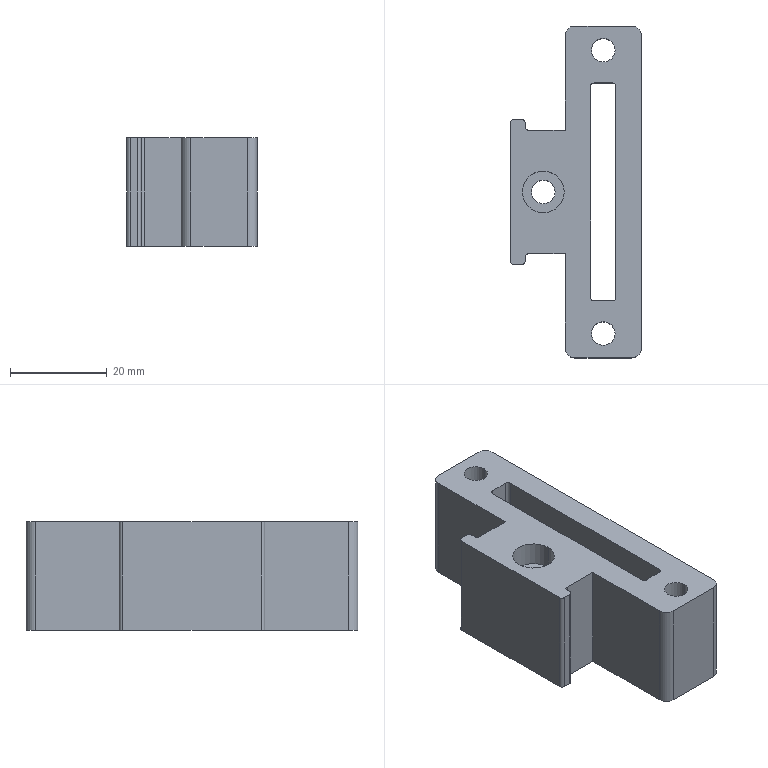Part | Creo | features DATUM PLANE 3, CURVE 2, COORDINATE SYSTEM 1, CUT 1, PROTRUSION 1, ROUND 1 | 1 solid | 41 faces | box 27 x 68.5 x 22.5 mm | volume 24185 mm3 | cylinder 22 | plane 19 | commonest cylinder face diameters 1.5 x10 4.88 x6 4 x4 8.617 x2
STEP:
#1=CARTESIAN_POINT('',(0.,0.,0.));
#2=DIRECTION('',(0.,0.,1.));
#3=DIRECTION('',(1.,0.,0.));
#4=AXIS2_PLACEMENT_3D('',#1,#2,#3);
#5=CARTESIAN_POINT('',(11.5,34.25,0.));
#6=VERTEX_POINT('',#5);
#7=CARTESIAN_POINT('',(13.5,32.25,0.));
#8=VERTEX_POINT('',#7);
#9=CARTESIAN_POINT('',(11.5,32.25,0.));
#10=DIRECTION('',(0.,0.,-1.));
#11=DIRECTION('',(0.,1.,0.));
#12=AXIS2_PLACEMENT_3D('',#9,#10,#11);
#13=CIRCLE('',#12,2.);
#14=EDGE_CURVE('',#6,#8,#13,.T.);
#15=ORIENTED_EDGE('',*,*,#14,.F.);
#16=CARTESIAN_POINT('',(-0.25,34.25,0.));
#17=VERTEX_POINT('',#16);
#18=CARTESIAN_POINT('',(11.5,34.25,0.));
#19=DIRECTION('',(-1.,0.,0.));
#20=VECTOR('',#19,11.75);
#21=LINE('',#18,#20);
#22=EDGE_CURVE('',#6,#17,#21,.T.);
#23=ORIENTED_EDGE('',*,*,#22,.T.);
#24=CARTESIAN_POINT('',(-2.25,32.25,0.));
#25=VERTEX_POINT('',#24);
#26=CARTESIAN_POINT('',(-0.25,32.25,0.));
#27=DIRECTION('',(0.,0.,-1.));
#28=DIRECTION('',(-1.,0.,0.));
#29=AXIS2_PLACEMENT_3D('',#26,#27,#28);
#30=CIRCLE('',#29,2.);
#31=EDGE_CURVE('',#25,#17,#30,.T.);
#32=ORIENTED_EDGE('',*,*,#31,.F.);
#33=CARTESIAN_POINT('',(-2.25,12.75,0.));
#34=VERTEX_POINT('',#33);
#35=CARTESIAN_POINT('',(-2.25,32.25,0.));
#36=DIRECTION('',(0.,-1.,0.));
#37=VECTOR('',#36,19.5);
#38=LINE('',#35,#37);
#39=EDGE_CURVE('',#25,#34,#38,.T.);
#40=ORIENTED_EDGE('',*,*,#39,.T.);
#41=CARTESIAN_POINT('',(-9.75,12.75,0.));
#42=VERTEX_POINT('',#41);
#43=CARTESIAN_POINT('',(-2.25,12.75,0.));
#44=DIRECTION('',(-1.,0.,0.));
#45=VECTOR('',#44,7.5);
#46=LINE('',#43,#45);
#47=EDGE_CURVE('',#34,#42,#46,.T.);
#48=ORIENTED_EDGE('',*,*,#47,.T.);
#49=CARTESIAN_POINT('',(-10.5,13.5,0.));
#50=VERTEX_POINT('',#49);
#51=CARTESIAN_POINT('',(-9.75,13.5,0.));
#52=DIRECTION('',(0.,0.,-1.));
#53=DIRECTION('',(0.,-1.,0.));
#54=AXIS2_PLACEMENT_3D('',#51,#52,#53);
#55=CIRCLE('',#54,0.75);
#56=EDGE_CURVE('',#42,#50,#55,.T.);
#57=ORIENTED_EDGE('',*,*,#56,.T.);
#58=CARTESIAN_POINT('',(-10.5,14.25,0.));
#59=VERTEX_POINT('',#58);
#60=CARTESIAN_POINT('',(-10.5,13.5,0.));
#61=DIRECTION('',(0.,1.,0.));
#62=VECTOR('',#61,0.75);
#63=LINE('',#60,#62);
#64=EDGE_CURVE('',#50,#59,#63,.T.);
#65=ORIENTED_EDGE('',*,*,#64,.T.);
#66=CARTESIAN_POINT('',(-11.25,15.,0.));
#67=VERTEX_POINT('',#66);
#68=CARTESIAN_POINT('',(-11.25,14.25,0.));
#69=DIRECTION('',(0.,0.,1.));
#70=DIRECTION('',(1.,0.,0.));
#71=AXIS2_PLACEMENT_3D('',#68,#69,#70);
#72=CIRCLE('',#71,0.75);
#73=EDGE_CURVE('',#59,#67,#72,.T.);
#74=ORIENTED_EDGE('',*,*,#73,.T.);
#75=CARTESIAN_POINT('',(-12.75,15.,0.));
#76=VERTEX_POINT('',#75);
#77=CARTESIAN_POINT('',(-11.25,15.,0.));
#78=DIRECTION('',(-1.,0.,0.));
#79=VECTOR('',#78,1.5);
#80=LINE('',#77,#79);
#81=EDGE_CURVE('',#67,#76,#80,.T.);
#82=ORIENTED_EDGE('',*,*,#81,.T.);
#83=CARTESIAN_POINT('',(-13.5,14.25,0.));
#84=VERTEX_POINT('',#83);
#85=CARTESIAN_POINT('',(-12.75,14.25,0.));
#86=DIRECTION('',(0.,0.,1.));
#87=DIRECTION('',(0.,1.,0.));
#88=AXIS2_PLACEMENT_3D('',#85,#86,#87);
#89=CIRCLE('',#88,0.75);
#90=EDGE_CURVE('',#76,#84,#89,.T.);
#91=ORIENTED_EDGE('',*,*,#90,.T.);
#92=CARTESIAN_POINT('',(-13.5,-14.25,0.));
#93=VERTEX_POINT('',#92);
#94=CARTESIAN_POINT('',(-13.5,14.25,0.));
#95=DIRECTION('',(0.,-1.,0.));
#96=VECTOR('',#95,28.5);
#97=LINE('',#94,#96);
#98=EDGE_CURVE('',#84,#93,#97,.T.);
#99=ORIENTED_EDGE('',*,*,#98,.T.);
#100=CARTESIAN_POINT('',(-12.75,-15.,0.));
#101=VERTEX_POINT('',#100);
#102=CARTESIAN_POINT('',(-12.75,-14.25,0.));
#103=DIRECTION('',(0.,0.,1.));
#104=DIRECTION('',(-1.,0.,0.));
#105=AXIS2_PLACEMENT_3D('',#102,#103,#104);
#106=CIRCLE('',#105,0.75);
#107=EDGE_CURVE('',#93,#101,#106,.T.);
#108=ORIENTED_EDGE('',*,*,#107,.T.);
#109=CARTESIAN_POINT('',(-11.25,-15.,0.));
#110=VERTEX_POINT('',#109);
#111=CARTESIAN_POINT('',(-12.75,-15.,0.));
#112=DIRECTION('',(1.,0.,0.));
#113=VECTOR('',#112,1.5);
#114=LINE('',#111,#113);
#115=EDGE_CURVE('',#101,#110,#114,.T.);
#116=ORIENTED_EDGE('',*,*,#115,.T.);
#117=CARTESIAN_POINT('',(-10.5,-14.25,0.));
#118=VERTEX_POINT('',#117);
#119=CARTESIAN_POINT('',(-11.25,-14.25,0.));
#120=DIRECTION('',(0.,0.,1.));
#121=DIRECTION('',(0.,-1.,0.));
#122=AXIS2_PLACEMENT_3D('',#119,#120,#121);
#123=CIRCLE('',#122,0.75);
#124=EDGE_CURVE('',#110,#118,#123,.T.);
#125=ORIENTED_EDGE('',*,*,#124,.T.);
#126=CARTESIAN_POINT('',(-10.5,-13.5,0.));
#127=VERTEX_POINT('',#126);
#128=CARTESIAN_POINT('',(-10.5,-14.25,0.));
#129=DIRECTION('',(0.,1.,0.));
#130=VECTOR('',#129,0.75);
#131=LINE('',#128,#130);
#132=EDGE_CURVE('',#118,#127,#131,.T.);
#133=ORIENTED_EDGE('',*,*,#132,.T.);
#134=CARTESIAN_POINT('',(-9.75,-12.75,0.));
#135=VERTEX_POINT('',#134);
#136=CARTESIAN_POINT('',(-9.75,-13.5,0.));
#137=DIRECTION('',(0.,0.,-1.));
#138=DIRECTION('',(-1.,0.,0.));
#139=AXIS2_PLACEMENT_3D('',#136,#137,#138);
#140=CIRCLE('',#139,0.75);
#141=EDGE_CURVE('',#127,#135,#140,.T.);
#142=ORIENTED_EDGE('',*,*,#141,.T.);
#143=CARTESIAN_POINT('',(-2.25,-12.75,0.));
#144=VERTEX_POINT('',#143);
#145=CARTESIAN_POINT('',(-9.75,-12.75,0.));
#146=DIRECTION('',(1.,0.,0.));
#147=VECTOR('',#146,7.5);
#148=LINE('',#145,#147);
#149=EDGE_CURVE('',#135,#144,#148,.T.);
#150=ORIENTED_EDGE('',*,*,#149,.T.);
#151=CARTESIAN_POINT('',(-2.25,-32.25,0.));
#152=VERTEX_POINT('',#151);
#153=CARTESIAN_POINT('',(-2.25,-12.75,0.));
#154=DIRECTION('',(0.,-1.,0.));
#155=VECTOR('',#154,19.5);
#156=LINE('',#153,#155);
#157=EDGE_CURVE('',#144,#152,#156,.T.);
#158=ORIENTED_EDGE('',*,*,#157,.T.);
#159=CARTESIAN_POINT('',(-0.25,-34.25,0.));
#160=VERTEX_POINT('',#159);
#161=CARTESIAN_POINT('',(-0.25,-32.25,0.));
#162=DIRECTION('',(0.,0.,-1.));
#163=DIRECTION('',(0.,-1.,0.));
#164=AXIS2_PLACEMENT_3D('',#161,#162,#163);
#165=CIRCLE('',#164,2.);
#166=EDGE_CURVE('',#160,#152,#165,.T.);
#167=ORIENTED_EDGE('',*,*,#166,.F.);
#168=CARTESIAN_POINT('',(11.5,-34.25,0.));
#169=VERTEX_POINT('',#168);
#170=CARTESIAN_POINT('',(-0.25,-34.25,0.));
#171=DIRECTION('',(1.,0.,0.));
#172=VECTOR('',#171,11.75);
#173=LINE('',#170,#172);
#174=EDGE_CURVE('',#160,#169,#173,.T.);
#175=ORIENTED_EDGE('',*,*,#174,.T.);
#176=CARTESIAN_POINT('',(13.5,-32.25,0.));
#177=VERTEX_POINT('',#176);
#178=CARTESIAN_POINT('',(11.5,-32.25,0.));
#179=DIRECTION('',(0.,0.,-1.));
#180=DIRECTION('',(1.,0.,0.));
#181=AXIS2_PLACEMENT_3D('',#178,#179,#180);
#182=CIRCLE('',#181,2.);
#183=EDGE_CURVE('',#177,#169,#182,.T.);
#184=ORIENTED_EDGE('',*,*,#183,.F.);
#185=CARTESIAN_POINT('',(13.5,-32.25,0.));
#186=DIRECTION('',(0.,1.,0.));
#187=VECTOR('',#186,64.5);
#188=LINE('',#185,#187);
#189=EDGE_CURVE('',#177,#8,#188,.T.);
#190=ORIENTED_EDGE('',*,*,#189,.T.);
#191=EDGE_LOOP('',(#15,#23,#32,#40,#48,#57,#65,#74,#82,#91,#99,#108,#116,#125,#133,#142,#150,#158,#167,#175,#184,#190));
#192=FACE_OUTER_BOUND('',#191,.F.);
#193=CARTESIAN_POINT('',(8.065,29.25,0.));
#194=VERTEX_POINT('',#193);
#195=CARTESIAN_POINT('',(3.185,29.25,0.));
#196=VERTEX_POINT('',#195);
#197=CARTESIAN_POINT('',(5.625,29.25,0.));
#198=DIRECTION('',(0.,0.,-1.));
#199=DIRECTION('',(1.,0.,0.));
#200=AXIS2_PLACEMENT_3D('',#197,#198,#199);
#201=CIRCLE('',#200,2.44);
#202=EDGE_CURVE('',#194,#196,#201,.T.);
#203=ORIENTED_EDGE('',*,*,#202,.T.);
#204=CARTESIAN_POINT('',(5.625,29.25,0.));
#205=DIRECTION('',(0.,0.,-1.));
#206=DIRECTION('',(-1.,0.,0.));
#207=AXIS2_PLACEMENT_3D('',#204,#205,#206);
#208=CIRCLE('',#207,2.44);
#209=EDGE_CURVE('',#196,#194,#208,.T.);
#210=ORIENTED_EDGE('',*,*,#209,.T.);
#211=EDGE_LOOP('',(#203,#210));
#212=FACE_BOUND('',#211,.F.);
#213=CARTESIAN_POINT('',(8.065,-29.25,0.));
#214=VERTEX_POINT('',#213);
#215=CARTESIAN_POINT('',(3.185,-29.25,0.));
#216=VERTEX_POINT('',#215);
#217=CARTESIAN_POINT('',(5.625,-29.25,0.));
#218=DIRECTION('',(0.,0.,-1.));
#219=DIRECTION('',(1.,0.,0.));
#220=AXIS2_PLACEMENT_3D('',#217,#218,#219);
#221=CIRCLE('',#220,2.44);
#222=EDGE_CURVE('',#214,#216,#221,.T.);
#223=ORIENTED_EDGE('',*,*,#222,.T.);
#224=CARTESIAN_POINT('',(5.625,-29.25,0.));
#225=DIRECTION('',(0.,0.,-1.));
#226=DIRECTION('',(-1.,0.,0.));
#227=AXIS2_PLACEMENT_3D('',#224,#225,#226);
#228=CIRCLE('',#227,2.44);
#229=EDGE_CURVE('',#216,#214,#228,.T.);
#230=ORIENTED_EDGE('',*,*,#229,.T.);
#231=EDGE_LOOP('',(#223,#230));
#232=FACE_BOUND('',#231,.F.);
#233=CARTESIAN_POINT('',(3.,21.75,0.));
#234=VERTEX_POINT('',#233);
#235=CARTESIAN_POINT('',(3.75,22.5,0.));
#236=VERTEX_POINT('',#235);
#237=CARTESIAN_POINT('',(3.75,21.75,0.));
#238=DIRECTION('',(0.,0.,-1.));
#239=DIRECTION('',(-1.,0.,0.));
#240=AXIS2_PLACEMENT_3D('',#237,#238,#239);
#241=CIRCLE('',#240,0.75);
#242=EDGE_CURVE('',#234,#236,#241,.T.);
#243=ORIENTED_EDGE('',*,*,#242,.T.);
#244=CARTESIAN_POINT('',(7.5,22.5,0.));
#245=VERTEX_POINT('',#244);
#246=CARTESIAN_POINT('',(3.75,22.5,0.));
#247=DIRECTION('',(1.,0.,0.));
#248=VECTOR('',#247,3.75);
#249=LINE('',#246,#248);
#250=EDGE_CURVE('',#236,#245,#249,.T.);
#251=ORIENTED_EDGE('',*,*,#250,.T.);
#252=CARTESIAN_POINT('',(8.25,21.75,0.));
#253=VERTEX_POINT('',#252);
#254=CARTESIAN_POINT('',(7.5,21.75,0.));
#255=DIRECTION('',(0.,0.,-1.));
#256=DIRECTION('',(0.,1.,0.));
#257=AXIS2_PLACEMENT_3D('',#254,#255,#256);
#258=CIRCLE('',#257,0.75);
#259=EDGE_CURVE('',#245,#253,#258,.T.);
#260=ORIENTED_EDGE('',*,*,#259,.T.);
#261=CARTESIAN_POINT('',(8.25,-21.75,0.));
#262=VERTEX_POINT('',#261);
#263=CARTESIAN_POINT('',(8.25,21.75,0.));
#264=DIRECTION('',(0.,-1.,0.));
#265=VECTOR('',#264,43.5);
#266=LINE('',#263,#265);
#267=EDGE_CURVE('',#253,#262,#266,.T.);
#268=ORIENTED_EDGE('',*,*,#267,.T.);
#269=CARTESIAN_POINT('',(7.5,-22.5,0.));
#270=VERTEX_POINT('',#269);
#271=CARTESIAN_POINT('',(7.5,-21.75,0.));
#272=DIRECTION('',(0.,0.,-1.));
#273=DIRECTION('',(1.,0.,0.));
#274=AXIS2_PLACEMENT_3D('',#271,#272,#273);
#275=CIRCLE('',#274,0.75);
#276=EDGE_CURVE('',#262,#270,#275,.T.);
#277=ORIENTED_EDGE('',*,*,#276,.T.);
#278=CARTESIAN_POINT('',(3.75,-22.5,0.));
#279=VERTEX_POINT('',#278);
#280=CARTESIAN_POINT('',(7.5,-22.5,0.));
#281=DIRECTION('',(-1.,0.,0.));
#282=VECTOR('',#281,3.75);
#283=LINE('',#280,#282);
#284=EDGE_CURVE('',#270,#279,#283,.T.);
#285=ORIENTED_EDGE('',*,*,#284,.T.);
#286=CARTESIAN_POINT('',(3.,-21.75,0.));
#287=VERTEX_POINT('',#286);
#288=CARTESIAN_POINT('',(3.75,-21.75,0.));
#289=DIRECTION('',(0.,0.,-1.));
#290=DIRECTION('',(0.,-1.,0.));
#291=AXIS2_PLACEMENT_3D('',#288,#289,#290);
#292=CIRCLE('',#291,0.75);
#293=EDGE_CURVE('',#279,#287,#292,.T.);
#294=ORIENTED_EDGE('',*,*,#293,.T.);
#295=CARTESIAN_POINT('',(3.,-21.75,0.));
#296=DIRECTION('',(0.,1.,0.));
#297=VECTOR('',#296,43.5);
#298=LINE('',#295,#297);
#299=EDGE_CURVE('',#287,#234,#298,.T.);
#300=ORIENTED_EDGE('',*,*,#299,.T.);
#301=EDGE_LOOP('',(#243,#251,#260,#268,#277,#285,#294,#300));
#302=FACE_BOUND('',#301,.F.);
#303=CARTESIAN_POINT('',(-4.31,0.,0.));
#304=VERTEX_POINT('',#303);
#305=CARTESIAN_POINT('',(-9.19,0.,0.));
#306=VERTEX_POINT('',#305);
#307=CARTESIAN_POINT('',(-6.75,0.,0.));
#308=DIRECTION('',(0.,0.,-1.));
#309=DIRECTION('',(1.,0.,0.));
#310=AXIS2_PLACEMENT_3D('',#307,#308,#309);
#311=CIRCLE('',#310,2.44);
#312=EDGE_CURVE('',#304,#306,#311,.T.);
#313=ORIENTED_EDGE('',*,*,#312,.T.);
#314=CARTESIAN_POINT('',(-6.75,0.,0.));
#315=DIRECTION('',(0.,0.,-1.));
#316=DIRECTION('',(-1.,0.,0.));
#317=AXIS2_PLACEMENT_3D('',#314,#315,#316);
#318=CIRCLE('',#317,2.44);
#319=EDGE_CURVE('',#306,#304,#318,.T.);
#320=ORIENTED_EDGE('',*,*,#319,.T.);
#321=EDGE_LOOP('',(#313,#320));
#322=FACE_BOUND('',#321,.F.);
#323=CARTESIAN_POINT('',(0.,0.,0.));
#324=DIRECTION('',(0.,0.,1.));
#325=DIRECTION('',(1.,0.,0.));
#326=AXIS2_PLACEMENT_3D('',#323,#324,#325);
#327=PLANE('',#326);
#328=ADVANCED_FACE('',(#192,#212,#232,#302,#322),#327,.F.);
#329=CARTESIAN_POINT('',(-9.19,0.,17.5));
#330=VERTEX_POINT('',#329);
#331=CARTESIAN_POINT('',(-4.31,0.,17.5));
#332=VERTEX_POINT('',#331);
#333=CARTESIAN_POINT('',(-6.75,0.,17.5));
#334=DIRECTION('',(0.,0.,1.));
#335=DIRECTION('',(-1.,0.,0.));
#336=AXIS2_PLACEMENT_3D('',#333,#334,#335);
#337=CIRCLE('',#336,2.44);
#338=EDGE_CURVE('',#330,#332,#337,.T.);
#339=ORIENTED_EDGE('',*,*,#338,.F.);
#340=CARTESIAN_POINT('',(-9.19,0.,0.));
#341=DIRECTION('',(0.,0.,1.));
#342=VECTOR('',#341,17.5);
#343=LINE('',#340,#342);
#344=EDGE_CURVE('',#306,#330,#343,.T.);
#345=ORIENTED_EDGE('',*,*,#344,.F.);
#346=ORIENTED_EDGE('',*,*,#312,.F.);
#347=CARTESIAN_POINT('',(-4.31,0.,0.));
#348=DIRECTION('',(0.,0.,1.));
#349=VECTOR('',#348,17.5);
#350=LINE('',#347,#349);
#351=EDGE_CURVE('',#304,#332,#350,.T.);
#352=ORIENTED_EDGE('',*,*,#351,.T.);
#353=EDGE_LOOP('',(#339,#345,#346,#352));
#354=FACE_OUTER_BOUND('',#353,.F.);
#355=CARTESIAN_POINT('',(-6.75,0.,0.));
#356=DIRECTION('',(0.,0.,1.));
#357=DIRECTION('',(1.,0.,0.));
#358=AXIS2_PLACEMENT_3D('',#355,#356,#357);
#359=CYLINDRICAL_SURFACE('',#358,2.44);
#360=ADVANCED_FACE('',(#354),#359,.F.);
#361=CARTESIAN_POINT('',(-2.441,0.,17.5));
#362=VERTEX_POINT('',#361);
#363=CARTESIAN_POINT('',(-11.059,0.,17.5));
#364=VERTEX_POINT('',#363);
#365=CARTESIAN_POINT('',(-6.75,0.,17.5));
#366=DIRECTION('',(0.,0.,1.));
#367=DIRECTION('',(1.,0.,0.));
#368=AXIS2_PLACEMENT_3D('',#365,#366,#367);
#369=CIRCLE('',#368,4.309);
#370=EDGE_CURVE('',#362,#364,#369,.T.);
#371=ORIENTED_EDGE('',*,*,#370,.F.);
#372=CARTESIAN_POINT('',(-6.75,0.,17.5));
#373=DIRECTION('',(0.,0.,1.));
#374=DIRECTION('',(-1.,0.,0.));
#375=AXIS2_PLACEMENT_3D('',#372,#373,#374);
#376=CIRCLE('',#375,4.309);
#377=EDGE_CURVE('',#364,#362,#376,.T.);
#378=ORIENTED_EDGE('',*,*,#377,.F.);
#379=EDGE_LOOP('',(#371,#378));
#380=FACE_OUTER_BOUND('',#379,.F.);
#381=ORIENTED_EDGE('',*,*,#338,.T.);
#382=CARTESIAN_POINT('',(-6.75,0.,17.5));
#383=DIRECTION('',(0.,0.,1.));
#384=DIRECTION('',(1.,0.,0.));
#385=AXIS2_PLACEMENT_3D('',#382,#383,#384);
#386=CIRCLE('',#385,2.44);
#387=EDGE_CURVE('',#332,#330,#386,.T.);
#388=ORIENTED_EDGE('',*,*,#387,.T.);
#389=EDGE_LOOP('',(#381,#388));
#390=FACE_BOUND('',#389,.F.);
#391=CARTESIAN_POINT('',(0.,0.,17.5));
#392=DIRECTION('',(0.,0.,1.));
#393=DIRECTION('',(1.,0.,0.));
#394=AXIS2_PLACEMENT_3D('',#391,#392,#393);
#395=PLANE('',#394);
#396=ADVANCED_FACE('',(#380,#390),#395,.T.);
#397=CARTESIAN_POINT('',(-2.441,0.,22.5));
#398=VERTEX_POINT('',#397);
#399=CARTESIAN_POINT('',(-11.059,0.,22.5));
#400=VERTEX_POINT('',#399);
#401=CARTESIAN_POINT('',(-6.75,0.,22.5));
#402=DIRECTION('',(0.,0.,1.));
#403=DIRECTION('',(1.,0.,0.));
#404=AXIS2_PLACEMENT_3D('',#401,#402,#403);
#405=CIRCLE('',#404,4.309);
#406=EDGE_CURVE('',#398,#400,#405,.T.);
#407=ORIENTED_EDGE('',*,*,#406,.F.);
#408=CARTESIAN_POINT('',(-2.441,0.,22.5));
#409=DIRECTION('',(0.,0.,-1.));
#410=VECTOR('',#409,5.);
#411=LINE('',#408,#410);
#412=EDGE_CURVE('',#398,#362,#411,.T.);
#413=ORIENTED_EDGE('',*,*,#412,.T.);
#414=ORIENTED_EDGE('',*,*,#370,.T.);
#415=CARTESIAN_POINT('',(-11.059,0.,22.5));
#416=DIRECTION('',(0.,0.,-1.));
#417=VECTOR('',#416,5.);
#418=LINE('',#415,#417);
#419=EDGE_CURVE('',#400,#364,#418,.T.);
#420=ORIENTED_EDGE('',*,*,#419,.F.);
#421=EDGE_LOOP('',(#407,#413,#414,#420));
#422=FACE_OUTER_BOUND('',#421,.F.);
#423=CARTESIAN_POINT('',(-6.75,0.,22.5));
#424=DIRECTION('',(0.,0.,1.));
#425=DIRECTION('',(1.,0.,0.));
#426=AXIS2_PLACEMENT_3D('',#423,#424,#425);
#427=CYLINDRICAL_SURFACE('',#426,4.309);
#428=ADVANCED_FACE('',(#422),#427,.F.);
#429=CARTESIAN_POINT('',(13.5,32.25,22.5));
#430=VERTEX_POINT('',#429);
#431=CARTESIAN_POINT('',(11.5,34.25,22.5));
#432=VERTEX_POINT('',#431);
#433=CARTESIAN_POINT('',(11.5,32.25,22.5));
#434=DIRECTION('',(0.,0.,1.));
#435=DIRECTION('',(1.,0.,0.));
#436=AXIS2_PLACEMENT_3D('',#433,#434,#435);
#437=CIRCLE('',#436,2.);
#438=EDGE_CURVE('',#430,#432,#437,.T.);
#439=ORIENTED_EDGE('',*,*,#438,.F.);
#440=CARTESIAN_POINT('',(13.5,-32.25,22.5));
#441=VERTEX_POINT('',#440);
#442=CARTESIAN_POINT('',(13.5,-32.25,22.5));
#443=DIRECTION('',(0.,1.,0.));
#444=VECTOR('',#443,64.5);
#445=LINE('',#442,#444);
#446=EDGE_CURVE('',#441,#430,#445,.T.);
#447=ORIENTED_EDGE('',*,*,#446,.F.);
#448=CARTESIAN_POINT('',(11.5,-34.25,22.5));
#449=VERTEX_POINT('',#448);
#450=CARTESIAN_POINT('',(11.5,-32.25,22.5));
#451=DIRECTION('',(0.,0.,1.));
#452=DIRECTION('',(0.,-1.,0.));
#453=AXIS2_PLACEMENT_3D('',#450,#451,#452);
#454=CIRCLE('',#453,2.);
#455=EDGE_CURVE('',#449,#441,#454,.T.);
#456=ORIENTED_EDGE('',*,*,#455,.F.);
#457=CARTESIAN_POINT('',(-0.25,-34.25,22.5));
#458=VERTEX_POINT('',#457);
#459=CARTESIAN_POINT('',(-0.25,-34.25,22.5));
#460=DIRECTION('',(1.,0.,0.));
#461=VECTOR('',#460,11.75);
#462=LINE('',#459,#461);
#463=EDGE_CURVE('',#458,#449,#462,.T.);
#464=ORIENTED_EDGE('',*,*,#463,.F.);
#465=CARTESIAN_POINT('',(-2.25,-32.25,22.5));
#466=VERTEX_POINT('',#465);
#467=CARTESIAN_POINT('',(-0.25,-32.25,22.5));
#468=DIRECTION('',(0.,0.,1.));
#469=DIRECTION('',(-1.,0.,0.));
#470=AXIS2_PLACEMENT_3D('',#467,#468,#469);
#471=CIRCLE('',#470,2.);
#472=EDGE_CURVE('',#466,#458,#471,.T.);
#473=ORIENTED_EDGE('',*,*,#472,.F.);
#474=CARTESIAN_POINT('',(-2.25,-12.75,22.5));
#475=VERTEX_POINT('',#474);
#476=CARTESIAN_POINT('',(-2.25,-12.75,22.5));
#477=DIRECTION('',(0.,-1.,0.));
#478=VECTOR('',#477,19.5);
#479=LINE('',#476,#478);
#480=EDGE_CURVE('',#475,#466,#479,.T.);
#481=ORIENTED_EDGE('',*,*,#480,.F.);
#482=CARTESIAN_POINT('',(-9.75,-12.75,22.5));
#483=VERTEX_POINT('',#482);
#484=CARTESIAN_POINT('',(-9.75,-12.75,22.5));
#485=DIRECTION('',(1.,0.,0.));
#486=VECTOR('',#485,7.5);
#487=LINE('',#484,#486);
#488=EDGE_CURVE('',#483,#475,#487,.T.);
#489=ORIENTED_EDGE('',*,*,#488,.F.);
#490=CARTESIAN_POINT('',(-10.5,-13.5,22.5));
#491=VERTEX_POINT('',#490);
#492=CARTESIAN_POINT('',(-9.75,-13.5,22.5));
#493=DIRECTION('',(0.,0.,-1.));
#494=DIRECTION('',(-1.,0.,0.));
#495=AXIS2_PLACEMENT_3D('',#492,#493,#494);
#496=CIRCLE('',#495,0.75);
#497=EDGE_CURVE('',#491,#483,#496,.T.);
#498=ORIENTED_EDGE('',*,*,#497,.F.);
#499=CARTESIAN_POINT('',(-10.5,-14.25,22.5));
#500=VERTEX_POINT('',#499);
#501=CARTESIAN_POINT('',(-10.5,-14.25,22.5));
#502=DIRECTION('',(0.,1.,0.));
#503=VECTOR('',#502,0.75);
#504=LINE('',#501,#503);
#505=EDGE_CURVE('',#500,#491,#504,.T.);
#506=ORIENTED_EDGE('',*,*,#505,.F.);
#507=CARTESIAN_POINT('',(-11.25,-15.,22.5));
#508=VERTEX_POINT('',#507);
#509=CARTESIAN_POINT('',(-11.25,-14.25,22.5));
#510=DIRECTION('',(0.,0.,1.));
#511=DIRECTION('',(0.,-1.,0.));
#512=AXIS2_PLACEMENT_3D('',#509,#510,#511);
#513=CIRCLE('',#512,0.75);
#514=EDGE_CURVE('',#508,#500,#513,.T.);
#515=ORIENTED_EDGE('',*,*,#514,.F.);
#516=CARTESIAN_POINT('',(-12.75,-15.,22.5));
#517=VERTEX_POINT('',#516);
#518=CARTESIAN_POINT('',(-12.75,-15.,22.5));
#519=DIRECTION('',(1.,0.,0.));
#520=VECTOR('',#519,1.5);
#521=LINE('',#518,#520);
#522=EDGE_CURVE('',#517,#508,#521,.T.);
#523=ORIENTED_EDGE('',*,*,#522,.F.);
#524=CARTESIAN_POINT('',(-13.5,-14.25,22.5));
#525=VERTEX_POINT('',#524);
#526=CARTESIAN_POINT('',(-12.75,-14.25,22.5));
#527=DIRECTION('',(0.,0.,1.));
#528=DIRECTION('',(-1.,0.,0.));
#529=AXIS2_PLACEMENT_3D('',#526,#527,#528);
#530=CIRCLE('',#529,0.75);
#531=EDGE_CURVE('',#525,#517,#530,.T.);
#532=ORIENTED_EDGE('',*,*,#531,.F.);
#533=CARTESIAN_POINT('',(-13.5,14.25,22.5));
#534=VERTEX_POINT('',#533);
#535=CARTESIAN_POINT('',(-13.5,14.25,22.5));
#536=DIRECTION('',(0.,-1.,0.));
#537=VECTOR('',#536,28.5);
#538=LINE('',#535,#537);
#539=EDGE_CURVE('',#534,#525,#538,.T.);
#540=ORIENTED_EDGE('',*,*,#539,.F.);
#541=CARTESIAN_POINT('',(-12.75,15.,22.5));
#542=VERTEX_POINT('',#541);
#543=CARTESIAN_POINT('',(-12.75,14.25,22.5));
#544=DIRECTION('',(0.,0.,1.));
#545=DIRECTION('',(0.,1.,0.));
#546=AXIS2_PLACEMENT_3D('',#543,#544,#545);
#547=CIRCLE('',#546,0.75);
#548=EDGE_CURVE('',#542,#534,#547,.T.);
#549=ORIENTED_EDGE('',*,*,#548,.F.);
#550=CARTESIAN_POINT('',(-11.25,15.,22.5));
#551=VERTEX_POINT('',#550);
#552=CARTESIAN_POINT('',(-11.25,15.,22.5));
#553=DIRECTION('',(-1.,0.,0.));
#554=VECTOR('',#553,1.5);
#555=LINE('',#552,#554);
#556=EDGE_CURVE('',#551,#542,#555,.T.);
#557=ORIENTED_EDGE('',*,*,#556,.F.);
#558=CARTESIAN_POINT('',(-10.5,14.25,22.5));
#559=VERTEX_POINT('',#558);
#560=CARTESIAN_POINT('',(-11.25,14.25,22.5));
#561=DIRECTION('',(0.,0.,1.));
#562=DIRECTION('',(1.,0.,0.));
#563=AXIS2_PLACEMENT_3D('',#560,#561,#562);
#564=CIRCLE('',#563,0.75);
#565=EDGE_CURVE('',#559,#551,#564,.T.);
#566=ORIENTED_EDGE('',*,*,#565,.F.);
#567=CARTESIAN_POINT('',(-10.5,13.5,22.5));
#568=VERTEX_POINT('',#567);
#569=CARTESIAN_POINT('',(-10.5,13.5,22.5));
#570=DIRECTION('',(0.,1.,0.));
#571=VECTOR('',#570,0.75);
#572=LINE('',#569,#571);
#573=EDGE_CURVE('',#568,#559,#572,.T.);
#574=ORIENTED_EDGE('',*,*,#573,.F.);
#575=CARTESIAN_POINT('',(-9.75,12.75,22.5));
#576=VERTEX_POINT('',#575);
#577=CARTESIAN_POINT('',(-9.75,13.5,22.5));
#578=DIRECTION('',(0.,0.,-1.));
#579=DIRECTION('',(0.,-1.,0.));
#580=AXIS2_PLACEMENT_3D('',#577,#578,#579);
#581=CIRCLE('',#580,0.75);
#582=EDGE_CURVE('',#576,#568,#581,.T.);
#583=ORIENTED_EDGE('',*,*,#582,.F.);
#584=CARTESIAN_POINT('',(-2.25,12.75,22.5));
#585=VERTEX_POINT('',#584);
#586=CARTESIAN_POINT('',(-2.25,12.75,22.5));
#587=DIRECTION('',(-1.,0.,0.));
#588=VECTOR('',#587,7.5);
#589=LINE('',#586,#588);
#590=EDGE_CURVE('',#585,#576,#589,.T.);
#591=ORIENTED_EDGE('',*,*,#590,.F.);
#592=CARTESIAN_POINT('',(-2.25,32.25,22.5));
#593=VERTEX_POINT('',#592);
#594=CARTESIAN_POINT('',(-2.25,32.25,22.5));
#595=DIRECTION('',(0.,-1.,0.));
#596=VECTOR('',#595,19.5);
#597=LINE('',#594,#596);
#598=EDGE_CURVE('',#593,#585,#597,.T.);
#599=ORIENTED_EDGE('',*,*,#598,.F.);
#600=CARTESIAN_POINT('',(-0.25,34.25,22.5));
#601=VERTEX_POINT('',#600);
#602=CARTESIAN_POINT('',(-0.25,32.25,22.5));
#603=DIRECTION('',(0.,0.,1.));
#604=DIRECTION('',(0.,1.,0.));
#605=AXIS2_PLACEMENT_3D('',#602,#603,#604);
#606=CIRCLE('',#605,2.);
#607=EDGE_CURVE('',#601,#593,#606,.T.);
#608=ORIENTED_EDGE('',*,*,#607,.F.);
#609=CARTESIAN_POINT('',(11.5,34.25,22.5));
#610=DIRECTION('',(-1.,0.,0.));
#611=VECTOR('',#610,11.75);
#612=LINE('',#609,#611);
#613=EDGE_CURVE('',#432,#601,#612,.T.);
#614=ORIENTED_EDGE('',*,*,#613,.F.);
#615=EDGE_LOOP('',(#439,#447,#456,#464,#473,#481,#489,#498,#506,#515,#523,#532,#540,#549,#557,#566,#574,#583,#591,#599,#608,#614));
#616=FACE_OUTER_BOUND('',#615,.F.);
#617=CARTESIAN_POINT('',(8.065,-29.25,22.5));
#618=VERTEX_POINT('',#617);
#619=CARTESIAN_POINT('',(3.185,-29.25,22.5));
#620=VERTEX_POINT('',#619);
#621=CARTESIAN_POINT('',(5.625,-29.25,22.5));
#622=DIRECTION('',(0.,0.,-1.));
#623=DIRECTION('',(1.,0.,0.));
#624=AXIS2_PLACEMENT_3D('',#621,#622,#623);
#625=CIRCLE('',#624,2.44);
#626=EDGE_CURVE('',#618,#620,#625,.T.);
#627=ORIENTED_EDGE('',*,*,#626,.F.);
#628=CARTESIAN_POINT('',(5.625,-29.25,22.5));
#629=DIRECTION('',(0.,0.,-1.));
#630=DIRECTION('',(-1.,0.,0.));
#631=AXIS2_PLACEMENT_3D('',#628,#629,#630);
#632=CIRCLE('',#631,2.44);
#633=EDGE_CURVE('',#620,#618,#632,.T.);
#634=ORIENTED_EDGE('',*,*,#633,.F.);
#635=EDGE_LOOP('',(#627,#634));
#636=FACE_BOUND('',#635,.F.);
#637=CARTESIAN_POINT('',(3.,21.75,22.5));
#638=VERTEX_POINT('',#637);
#639=CARTESIAN_POINT('',(3.75,22.5,22.5));
#640=VERTEX_POINT('',#639);
#641=CARTESIAN_POINT('',(3.75,21.75,22.5));
#642=DIRECTION('',(0.,0.,-1.));
#643=DIRECTION('',(-1.,0.,0.));
#644=AXIS2_PLACEMENT_3D('',#641,#642,#643);
#645=CIRCLE('',#644,0.75);
#646=EDGE_CURVE('',#638,#640,#645,.T.);
#647=ORIENTED_EDGE('',*,*,#646,.F.);
#648=CARTESIAN_POINT('',(3.,-21.75,22.5));
#649=VERTEX_POINT('',#648);
#650=CARTESIAN_POINT('',(3.,-21.75,22.5));
#651=DIRECTION('',(0.,1.,0.));
#652=VECTOR('',#651,43.5);
#653=LINE('',#650,#652);
#654=EDGE_CURVE('',#649,#638,#653,.T.);
#655=ORIENTED_EDGE('',*,*,#654,.F.);
#656=CARTESIAN_POINT('',(3.75,-22.5,22.5));
#657=VERTEX_POINT('',#656);
#658=CARTESIAN_POINT('',(3.75,-21.75,22.5));
#659=DIRECTION('',(0.,0.,-1.));
#660=DIRECTION('',(0.,-1.,0.));
#661=AXIS2_PLACEMENT_3D('',#658,#659,#660);
#662=CIRCLE('',#661,0.75);
#663=EDGE_CURVE('',#657,#649,#662,.T.);
#664=ORIENTED_EDGE('',*,*,#663,.F.);
#665=CARTESIAN_POINT('',(7.5,-22.5,22.5));
#666=VERTEX_POINT('',#665);
#667=CARTESIAN_POINT('',(7.5,-22.5,22.5));
#668=DIRECTION('',(-1.,0.,0.));
#669=VECTOR('',#668,3.75);
#670=LINE('',#667,#669);
#671=EDGE_CURVE('',#666,#657,#670,.T.);
#672=ORIENTED_EDGE('',*,*,#671,.F.);
#673=CARTESIAN_POINT('',(8.25,-21.75,22.5));
#674=VERTEX_POINT('',#673);
#675=CARTESIAN_POINT('',(7.5,-21.75,22.5));
#676=DIRECTION('',(0.,0.,-1.));
#677=DIRECTION('',(1.,0.,0.));
#678=AXIS2_PLACEMENT_3D('',#675,#676,#677);
#679=CIRCLE('',#678,0.75);
#680=EDGE_CURVE('',#674,#666,#679,.T.);
#681=ORIENTED_EDGE('',*,*,#680,.F.);
#682=CARTESIAN_POINT('',(8.25,21.75,22.5));
#683=VERTEX_POINT('',#682);
#684=CARTESIAN_POINT('',(8.25,21.75,22.5));
#685=DIRECTION('',(0.,-1.,0.));
#686=VECTOR('',#685,43.5);
#687=LINE('',#684,#686);
#688=EDGE_CURVE('',#683,#674,#687,.T.);
#689=ORIENTED_EDGE('',*,*,#688,.F.);
#690=CARTESIAN_POINT('',(7.5,22.5,22.5));
#691=VERTEX_POINT('',#690);
#692=CARTESIAN_POINT('',(7.5,21.75,22.5));
#693=DIRECTION('',(0.,0.,-1.));
#694=DIRECTION('',(0.,1.,0.));
#695=AXIS2_PLACEMENT_3D('',#692,#693,#694);
#696=CIRCLE('',#695,0.75);
#697=EDGE_CURVE('',#691,#683,#696,.T.);
#698=ORIENTED_EDGE('',*,*,#697,.F.);
#699=CARTESIAN_POINT('',(3.75,22.5,22.5));
#700=DIRECTION('',(1.,0.,0.));
#701=VECTOR('',#700,3.75);
#702=LINE('',#699,#701);
#703=EDGE_CURVE('',#640,#691,#702,.T.);
#704=ORIENTED_EDGE('',*,*,#703,.F.);
#705=EDGE_LOOP('',(#647,#655,#664,#672,#681,#689,#698,#704));
#706=FACE_BOUND('',#705,.F.);
#707=ORIENTED_EDGE('',*,*,#406,.T.);
#708=CARTESIAN_POINT('',(-6.75,0.,22.5));
#709=DIRECTION('',(0.,0.,1.));
#710=DIRECTION('',(-1.,0.,0.));
#711=AXIS2_PLACEMENT_3D('',#708,#709,#710);
#712=CIRCLE('',#711,4.309);
#713=EDGE_CURVE('',#400,#398,#712,.T.);
#714=ORIENTED_EDGE('',*,*,#713,.T.);
#715=EDGE_LOOP('',(#707,#714));
#716=FACE_BOUND('',#715,.F.);
#717=CARTESIAN_POINT('',(8.065,29.25,22.5));
#718=VERTEX_POINT('',#717);
#719=CARTESIAN_POINT('',(3.185,29.25,22.5));
#720=VERTEX_POINT('',#719);
#721=CARTESIAN_POINT('',(5.625,29.25,22.5));
#722=DIRECTION('',(0.,0.,-1.));
#723=DIRECTION('',(1.,0.,0.));
#724=AXIS2_PLACEMENT_3D('',#721,#722,#723);
#725=CIRCLE('',#724,2.44);
#726=EDGE_CURVE('',#718,#720,#725,.T.);
#727=ORIENTED_EDGE('',*,*,#726,.F.);
#728=CARTESIAN_POINT('',(5.625,29.25,22.5));
#729=DIRECTION('',(0.,0.,-1.));
#730=DIRECTION('',(-1.,0.,0.));
#731=AXIS2_PLACEMENT_3D('',#728,#729,#730);
#732=CIRCLE('',#731,2.44);
#733=EDGE_CURVE('',#720,#718,#732,.T.);
#734=ORIENTED_EDGE('',*,*,#733,.F.);
#735=EDGE_LOOP('',(#727,#734));
#736=FACE_BOUND('',#735,.F.);
#737=CARTESIAN_POINT('',(0.,0.,22.5));
#738=DIRECTION('',(0.,0.,1.));
#739=DIRECTION('',(1.,0.,0.));
#740=AXIS2_PLACEMENT_3D('',#737,#738,#739);
#741=PLANE('',#740);
#742=ADVANCED_FACE('',(#616,#636,#706,#716,#736),#741,.T.);
#743=ORIENTED_EDGE('',*,*,#202,.F.);
#744=CARTESIAN_POINT('',(8.065,29.25,0.));
#745=DIRECTION('',(0.,0.,1.));
#746=VECTOR('',#745,22.5);
#747=LINE('',#744,#746);
#748=EDGE_CURVE('',#194,#718,#747,.T.);
#749=ORIENTED_EDGE('',*,*,#748,.T.);
#750=ORIENTED_EDGE('',*,*,#726,.T.);
#751=CARTESIAN_POINT('',(3.185,29.25,0.));
#752=DIRECTION('',(0.,0.,1.));
#753=VECTOR('',#752,22.5);
#754=LINE('',#751,#753);
#755=EDGE_CURVE('',#196,#720,#754,.T.);
#756=ORIENTED_EDGE('',*,*,#755,.F.);
#757=EDGE_LOOP('',(#743,#749,#750,#756));
#758=FACE_OUTER_BOUND('',#757,.F.);
#759=CARTESIAN_POINT('',(5.625,29.25,0.));
#760=DIRECTION('',(0.,0.,1.));
#761=DIRECTION('',(1.,0.,0.));
#762=AXIS2_PLACEMENT_3D('',#759,#760,#761);
#763=CYLINDRICAL_SURFACE('',#762,2.44);
#764=ADVANCED_FACE('',(#758),#763,.F.);
#765=ORIENTED_EDGE('',*,*,#209,.F.);
#766=ORIENTED_EDGE('',*,*,#755,.T.);
#767=ORIENTED_EDGE('',*,*,#733,.T.);
#768=ORIENTED_EDGE('',*,*,#748,.F.);
#769=EDGE_LOOP('',(#765,#766,#767,#768));
#770=FACE_OUTER_BOUND('',#769,.F.);
#771=CARTESIAN_POINT('',(5.625,29.25,0.));
#772=DIRECTION('',(0.,0.,1.));
#773=DIRECTION('',(1.,0.,0.));
#774=AXIS2_PLACEMENT_3D('',#771,#772,#773);
#775=CYLINDRICAL_SURFACE('',#774,2.44);
#776=ADVANCED_FACE('',(#770),#775,.F.);
#777=ORIENTED_EDGE('',*,*,#222,.F.);
#778=CARTESIAN_POINT('',(8.065,-29.25,0.));
#779=DIRECTION('',(0.,0.,1.));
#780=VECTOR('',#779,22.5);
#781=LINE('',#778,#780);
#782=EDGE_CURVE('',#214,#618,#781,.T.);
#783=ORIENTED_EDGE('',*,*,#782,.T.);
#784=ORIENTED_EDGE('',*,*,#626,.T.);
#785=CARTESIAN_POINT('',(3.185,-29.25,0.));
#786=DIRECTION('',(0.,0.,1.));
#787=VECTOR('',#786,22.5);
#788=LINE('',#785,#787);
#789=EDGE_CURVE('',#216,#620,#788,.T.);
#790=ORIENTED_EDGE('',*,*,#789,.F.);
#791=EDGE_LOOP('',(#777,#783,#784,#790));
#792=FACE_OUTER_BOUND('',#791,.F.);
#793=CARTESIAN_POINT('',(5.625,-29.25,0.));
#794=DIRECTION('',(0.,0.,1.));
#795=DIRECTION('',(1.,0.,0.));
#796=AXIS2_PLACEMENT_3D('',#793,#794,#795);
#797=CYLINDRICAL_SURFACE('',#796,2.44);
#798=ADVANCED_FACE('',(#792),#797,.F.);
#799=ORIENTED_EDGE('',*,*,#229,.F.);
#800=ORIENTED_EDGE('',*,*,#789,.T.);
#801=ORIENTED_EDGE('',*,*,#633,.T.);
#802=ORIENTED_EDGE('',*,*,#782,.F.);
#803=EDGE_LOOP('',(#799,#800,#801,#802));
#804=FACE_OUTER_BOUND('',#803,.F.);
#805=CARTESIAN_POINT('',(5.625,-29.25,0.));
#806=DIRECTION('',(0.,0.,1.));
#807=DIRECTION('',(1.,0.,0.));
#808=AXIS2_PLACEMENT_3D('',#805,#806,#807);
#809=CYLINDRICAL_SURFACE('',#808,2.44);
#810=ADVANCED_FACE('',(#804),#809,.F.);
#811=ORIENTED_EDGE('',*,*,#242,.F.);
#812=CARTESIAN_POINT('',(3.,21.75,0.));
#813=DIRECTION('',(0.,0.,1.));
#814=VECTOR('',#813,22.5);
#815=LINE('',#812,#814);
#816=EDGE_CURVE('',#234,#638,#815,.T.);
#817=ORIENTED_EDGE('',*,*,#816,.T.);
#818=ORIENTED_EDGE('',*,*,#646,.T.);
#819=CARTESIAN_POINT('',(3.75,22.5,0.));
#820=DIRECTION('',(0.,0.,1.));
#821=VECTOR('',#820,22.5);
#822=LINE('',#819,#821);
#823=EDGE_CURVE('',#236,#640,#822,.T.);
#824=ORIENTED_EDGE('',*,*,#823,.F.);
#825=EDGE_LOOP('',(#811,#817,#818,#824));
#826=FACE_OUTER_BOUND('',#825,.F.);
#827=CARTESIAN_POINT('',(3.75,21.75,0.));
#828=DIRECTION('',(0.,0.,1.));
#829=DIRECTION('',(1.,0.,0.));
#830=AXIS2_PLACEMENT_3D('',#827,#828,#829);
#831=CYLINDRICAL_SURFACE('',#830,0.75);
#832=ADVANCED_FACE('',(#826),#831,.F.);
#833=ORIENTED_EDGE('',*,*,#299,.F.);
#834=CARTESIAN_POINT('',(3.,-21.75,0.));
#835=DIRECTION('',(0.,0.,1.));
#836=VECTOR('',#835,22.5);
#837=LINE('',#834,#836);
#838=EDGE_CURVE('',#287,#649,#837,.T.);
#839=ORIENTED_EDGE('',*,*,#838,.T.);
#840=ORIENTED_EDGE('',*,*,#654,.T.);
#841=ORIENTED_EDGE('',*,*,#816,.F.);
#842=EDGE_LOOP('',(#833,#839,#840,#841));
#843=FACE_OUTER_BOUND('',#842,.F.);
#844=CARTESIAN_POINT('',(3.,-21.75,0.));
#845=DIRECTION('',(1.,0.,0.));
#846=DIRECTION('',(0.,1.,0.));
#847=AXIS2_PLACEMENT_3D('',#844,#845,#846);
#848=PLANE('',#847);
#849=ADVANCED_FACE('',(#843),#848,.T.);
#850=ORIENTED_EDGE('',*,*,#293,.F.);
#851=CARTESIAN_POINT('',(3.75,-22.5,0.));
#852=DIRECTION('',(0.,0.,1.));
#853=VECTOR('',#852,22.5);
#854=LINE('',#851,#853);
#855=EDGE_CURVE('',#279,#657,#854,.T.);
#856=ORIENTED_EDGE('',*,*,#855,.T.);
#857=ORIENTED_EDGE('',*,*,#663,.T.);
#858=ORIENTED_EDGE('',*,*,#838,.F.);
#859=EDGE_LOOP('',(#850,#856,#857,#858));
#860=FACE_OUTER_BOUND('',#859,.F.);
#861=CARTESIAN_POINT('',(3.75,-21.75,0.));
#862=DIRECTION('',(0.,0.,1.));
#863=DIRECTION('',(1.,0.,0.));
#864=AXIS2_PLACEMENT_3D('',#861,#862,#863);
#865=CYLINDRICAL_SURFACE('',#864,0.75);
#866=ADVANCED_FACE('',(#860),#865,.F.);
#867=ORIENTED_EDGE('',*,*,#284,.F.);
#868=CARTESIAN_POINT('',(7.5,-22.5,0.));
#869=DIRECTION('',(0.,0.,1.));
#870=VECTOR('',#869,22.5);
#871=LINE('',#868,#870);
#872=EDGE_CURVE('',#270,#666,#871,.T.);
#873=ORIENTED_EDGE('',*,*,#872,.T.);
#874=ORIENTED_EDGE('',*,*,#671,.T.);
#875=ORIENTED_EDGE('',*,*,#855,.F.);
#876=EDGE_LOOP('',(#867,#873,#874,#875));
#877=FACE_OUTER_BOUND('',#876,.F.);
#878=CARTESIAN_POINT('',(7.5,-22.5,0.));
#879=DIRECTION('',(0.,1.,0.));
#880=DIRECTION('',(-1.,0.,0.));
#881=AXIS2_PLACEMENT_3D('',#878,#879,#880);
#882=PLANE('',#881);
#883=ADVANCED_FACE('',(#877),#882,.T.);
#884=ORIENTED_EDGE('',*,*,#276,.F.);
#885=CARTESIAN_POINT('',(8.25,-21.75,0.));
#886=DIRECTION('',(0.,0.,1.));
#887=VECTOR('',#886,22.5);
#888=LINE('',#885,#887);
#889=EDGE_CURVE('',#262,#674,#888,.T.);
#890=ORIENTED_EDGE('',*,*,#889,.T.);
#891=ORIENTED_EDGE('',*,*,#680,.T.);
#892=ORIENTED_EDGE('',*,*,#872,.F.);
#893=EDGE_LOOP('',(#884,#890,#891,#892));
#894=FACE_OUTER_BOUND('',#893,.F.);
#895=CARTESIAN_POINT('',(7.5,-21.75,0.));
#896=DIRECTION('',(0.,0.,1.));
#897=DIRECTION('',(1.,0.,0.));
#898=AXIS2_PLACEMENT_3D('',#895,#896,#897);
#899=CYLINDRICAL_SURFACE('',#898,0.75);
#900=ADVANCED_FACE('',(#894),#899,.F.);
#901=ORIENTED_EDGE('',*,*,#267,.F.);
#902=CARTESIAN_POINT('',(8.25,21.75,0.));
#903=DIRECTION('',(0.,0.,1.));
#904=VECTOR('',#903,22.5);
#905=LINE('',#902,#904);
#906=EDGE_CURVE('',#253,#683,#905,.T.);
#907=ORIENTED_EDGE('',*,*,#906,.T.);
#908=ORIENTED_EDGE('',*,*,#688,.T.);
#909=ORIENTED_EDGE('',*,*,#889,.F.);
#910=EDGE_LOOP('',(#901,#907,#908,#909));
#911=FACE_OUTER_BOUND('',#910,.F.);
#912=CARTESIAN_POINT('',(8.25,21.75,0.));
#913=DIRECTION('',(-1.,0.,0.));
#914=DIRECTION('',(0.,-1.,0.));
#915=AXIS2_PLACEMENT_3D('',#912,#913,#914);
#916=PLANE('',#915);
#917=ADVANCED_FACE('',(#911),#916,.T.);
#918=ORIENTED_EDGE('',*,*,#259,.F.);
#919=CARTESIAN_POINT('',(7.5,22.5,0.));
#920=DIRECTION('',(0.,0.,1.));
#921=VECTOR('',#920,22.5);
#922=LINE('',#919,#921);
#923=EDGE_CURVE('',#245,#691,#922,.T.);
#924=ORIENTED_EDGE('',*,*,#923,.T.);
#925=ORIENTED_EDGE('',*,*,#697,.T.);
#926=ORIENTED_EDGE('',*,*,#906,.F.);
#927=EDGE_LOOP('',(#918,#924,#925,#926));
#928=FACE_OUTER_BOUND('',#927,.F.);
#929=CARTESIAN_POINT('',(7.5,21.75,0.));
#930=DIRECTION('',(0.,0.,1.));
#931=DIRECTION('',(1.,0.,0.));
#932=AXIS2_PLACEMENT_3D('',#929,#930,#931);
#933=CYLINDRICAL_SURFACE('',#932,0.75);
#934=ADVANCED_FACE('',(#928),#933,.F.);
#935=ORIENTED_EDGE('',*,*,#250,.F.);
#936=ORIENTED_EDGE('',*,*,#823,.T.);
#937=ORIENTED_EDGE('',*,*,#703,.T.);
#938=ORIENTED_EDGE('',*,*,#923,.F.);
#939=EDGE_LOOP('',(#935,#936,#937,#938));
#940=FACE_OUTER_BOUND('',#939,.F.);
#941=CARTESIAN_POINT('',(3.75,22.5,0.));
#942=DIRECTION('',(0.,-1.,0.));
#943=DIRECTION('',(1.,0.,0.));
#944=AXIS2_PLACEMENT_3D('',#941,#942,#943);
#945=PLANE('',#944);
#946=ADVANCED_FACE('',(#940),#945,.T.);
#947=ORIENTED_EDGE('',*,*,#713,.F.);
#948=ORIENTED_EDGE('',*,*,#419,.T.);
#949=ORIENTED_EDGE('',*,*,#377,.T.);
#950=ORIENTED_EDGE('',*,*,#412,.F.);
#951=EDGE_LOOP('',(#947,#948,#949,#950));
#952=FACE_OUTER_BOUND('',#951,.F.);
#953=CARTESIAN_POINT('',(-6.75,0.,22.5));
#954=DIRECTION('',(0.,0.,1.));
#955=DIRECTION('',(1.,0.,0.));
#956=AXIS2_PLACEMENT_3D('',#953,#954,#955);
#957=CYLINDRICAL_SURFACE('',#956,4.309);
#958=ADVANCED_FACE('',(#952),#957,.F.);
#959=ORIENTED_EDGE('',*,*,#14,.T.);
#960=CARTESIAN_POINT('',(13.5,32.25,22.5));
#961=DIRECTION('',(0.,0.,-1.));
#962=VECTOR('',#961,22.5);
#963=LINE('',#960,#962);
#964=EDGE_CURVE('',#430,#8,#963,.T.);
#965=ORIENTED_EDGE('',*,*,#964,.F.);
#966=ORIENTED_EDGE('',*,*,#438,.T.);
#967=CARTESIAN_POINT('',(11.5,34.25,22.5));
#968=DIRECTION('',(0.,0.,-1.));
#969=VECTOR('',#968,22.5);
#970=LINE('',#967,#969);
#971=EDGE_CURVE('',#432,#6,#970,.T.);
#972=ORIENTED_EDGE('',*,*,#971,.T.);
#973=EDGE_LOOP('',(#959,#965,#966,#972));
#974=FACE_OUTER_BOUND('',#973,.F.);
#975=CARTESIAN_POINT('',(11.5,32.25,51.831));
#976=DIRECTION('',(0.,0.,-1.));
#977=DIRECTION('',(0.,1.,0.));
#978=AXIS2_PLACEMENT_3D('',#975,#976,#977);
#979=CYLINDRICAL_SURFACE('',#978,2.);
#980=ADVANCED_FACE('',(#974),#979,.T.);
#981=ORIENTED_EDGE('',*,*,#964,.T.);
#982=ORIENTED_EDGE('',*,*,#189,.F.);
#983=CARTESIAN_POINT('',(13.5,-32.25,22.5));
#984=DIRECTION('',(0.,0.,-1.));
#985=VECTOR('',#984,22.5);
#986=LINE('',#983,#985);
#987=EDGE_CURVE('',#441,#177,#986,.T.);
#988=ORIENTED_EDGE('',*,*,#987,.F.);
#989=ORIENTED_EDGE('',*,*,#446,.T.);
#990=EDGE_LOOP('',(#981,#982,#988,#989));
#991=FACE_OUTER_BOUND('',#990,.F.);
#992=CARTESIAN_POINT('',(13.5,-34.25,0.));
#993=DIRECTION('',(1.,0.,0.));
#994=DIRECTION('',(0.,1.,0.));
#995=AXIS2_PLACEMENT_3D('',#992,#993,#994);
#996=PLANE('',#995);
#997=ADVANCED_FACE('',(#991),#996,.T.);
#998=ORIENTED_EDGE('',*,*,#183,.T.);
#999=CARTESIAN_POINT('',(11.5,-34.25,22.5));
#1000=DIRECTION('',(0.,0.,-1.));
#1001=VECTOR('',#1000,22.5);
#1002=LINE('',#999,#1001);
#1003=EDGE_CURVE('',#449,#169,#1002,.T.);
#1004=ORIENTED_EDGE('',*,*,#1003,.F.);
#1005=ORIENTED_EDGE('',*,*,#455,.T.);
#1006=ORIENTED_EDGE('',*,*,#987,.T.);
#1007=EDGE_LOOP('',(#998,#1004,#1005,#1006));
#1008=FACE_OUTER_BOUND('',#1007,.F.);
#1009=CARTESIAN_POINT('',(11.5,-32.25,51.831));
#1010=DIRECTION('',(0.,0.,-1.));
#1011=DIRECTION('',(1.,0.,0.));
#1012=AXIS2_PLACEMENT_3D('',#1009,#1010,#1011);
#1013=CYLINDRICAL_SURFACE('',#1012,2.);
#1014=ADVANCED_FACE('',(#1008),#1013,.T.);
#1015=CARTESIAN_POINT('',(-0.25,-34.25,22.5));
#1016=DIRECTION('',(0.,0.,-1.));
#1017=VECTOR('',#1016,22.5);
#1018=LINE('',#1015,#1017);
#1019=EDGE_CURVE('',#458,#160,#1018,.T.);
#1020=ORIENTED_EDGE('',*,*,#1019,.F.);
#1021=ORIENTED_EDGE('',*,*,#463,.T.);
#1022=ORIENTED_EDGE('',*,*,#1003,.T.);
#1023=ORIENTED_EDGE('',*,*,#174,.F.);
#1024=EDGE_LOOP('',(#1020,#1021,#1022,#1023));
#1025=FACE_OUTER_BOUND('',#1024,.F.);
#1026=CARTESIAN_POINT('',(-2.25,-34.25,0.));
#1027=DIRECTION('',(0.,-1.,0.));
#1028=DIRECTION('',(1.,0.,0.));
#1029=AXIS2_PLACEMENT_3D('',#1026,#1027,#1028);
#1030=PLANE('',#1029);
#1031=ADVANCED_FACE('',(#1025),#1030,.T.);
#1032=ORIENTED_EDGE('',*,*,#166,.T.);
#1033=CARTESIAN_POINT('',(-2.25,-32.25,22.5));
#1034=DIRECTION('',(0.,0.,-1.));
#1035=VECTOR('',#1034,22.5);
#1036=LINE('',#1033,#1035);
#1037=EDGE_CURVE('',#466,#152,#1036,.T.);
#1038=ORIENTED_EDGE('',*,*,#1037,.F.);
#1039=ORIENTED_EDGE('',*,*,#472,.T.);
#1040=ORIENTED_EDGE('',*,*,#1019,.T.);
#1041=EDGE_LOOP('',(#1032,#1038,#1039,#1040));
#1042=FACE_OUTER_BOUND('',#1041,.F.);
#1043=CARTESIAN_POINT('',(-0.25,-32.25,51.831));
#1044=DIRECTION('',(0.,0.,-1.));
#1045=DIRECTION('',(0.,-1.,0.));
#1046=AXIS2_PLACEMENT_3D('',#1043,#1044,#1045);
#1047=CYLINDRICAL_SURFACE('',#1046,2.);
#1048=ADVANCED_FACE('',(#1042),#1047,.T.);
#1049=ORIENTED_EDGE('',*,*,#1037,.T.);
#1050=ORIENTED_EDGE('',*,*,#157,.F.);
#1051=CARTESIAN_POINT('',(-2.25,-12.75,0.));
#1052=DIRECTION('',(0.,0.,1.));
#1053=VECTOR('',#1052,22.5);
#1054=LINE('',#1051,#1053);
#1055=EDGE_CURVE('',#144,#475,#1054,.T.);
#1056=ORIENTED_EDGE('',*,*,#1055,.T.);
#1057=ORIENTED_EDGE('',*,*,#480,.T.);
#1058=EDGE_LOOP('',(#1049,#1050,#1056,#1057));
#1059=FACE_OUTER_BOUND('',#1058,.F.);
#1060=CARTESIAN_POINT('',(-2.25,-12.75,0.));
#1061=DIRECTION('',(-1.,0.,0.));
#1062=DIRECTION('',(0.,-1.,0.));
#1063=AXIS2_PLACEMENT_3D('',#1060,#1061,#1062);
#1064=PLANE('',#1063);
#1065=ADVANCED_FACE('',(#1059),#1064,.T.);
#1066=ORIENTED_EDGE('',*,*,#149,.F.);
#1067=CARTESIAN_POINT('',(-9.75,-12.75,0.));
#1068=DIRECTION('',(0.,0.,1.));
#1069=VECTOR('',#1068,22.5);
#1070=LINE('',#1067,#1069);
#1071=EDGE_CURVE('',#135,#483,#1070,.T.);
#1072=ORIENTED_EDGE('',*,*,#1071,.T.);
#1073=ORIENTED_EDGE('',*,*,#488,.T.);
#1074=ORIENTED_EDGE('',*,*,#1055,.F.);
#1075=EDGE_LOOP('',(#1066,#1072,#1073,#1074));
#1076=FACE_OUTER_BOUND('',#1075,.F.);
#1077=CARTESIAN_POINT('',(-9.75,-12.75,0.));
#1078=DIRECTION('',(0.,-1.,0.));
#1079=DIRECTION('',(1.,0.,0.));
#1080=AXIS2_PLACEMENT_3D('',#1077,#1078,#1079);
#1081=PLANE('',#1080);
#1082=ADVANCED_FACE('',(#1076),#1081,.T.);
#1083=ORIENTED_EDGE('',*,*,#141,.F.);
#1084=CARTESIAN_POINT('',(-10.5,-13.5,0.));
#1085=DIRECTION('',(0.,0.,1.));
#1086=VECTOR('',#1085,22.5);
#1087=LINE('',#1084,#1086);
#1088=EDGE_CURVE('',#127,#491,#1087,.T.);
#1089=ORIENTED_EDGE('',*,*,#1088,.T.);
#1090=ORIENTED_EDGE('',*,*,#497,.T.);
#1091=ORIENTED_EDGE('',*,*,#1071,.F.);
#1092=EDGE_LOOP('',(#1083,#1089,#1090,#1091));
#1093=FACE_OUTER_BOUND('',#1092,.F.);
#1094=CARTESIAN_POINT('',(-9.75,-13.5,0.));
#1095=DIRECTION('',(0.,0.,1.));
#1096=DIRECTION('',(1.,0.,0.));
#1097=AXIS2_PLACEMENT_3D('',#1094,#1095,#1096);
#1098=CYLINDRICAL_SURFACE('',#1097,0.75);
#1099=ADVANCED_FACE('',(#1093),#1098,.F.);
#1100=ORIENTED_EDGE('',*,*,#132,.F.);
#1101=CARTESIAN_POINT('',(-10.5,-14.25,0.));
#1102=DIRECTION('',(0.,0.,1.));
#1103=VECTOR('',#1102,22.5);
#1104=LINE('',#1101,#1103);
#1105=EDGE_CURVE('',#118,#500,#1104,.T.);
#1106=ORIENTED_EDGE('',*,*,#1105,.T.);
#1107=ORIENTED_EDGE('',*,*,#505,.T.);
#1108=ORIENTED_EDGE('',*,*,#1088,.F.);
#1109=EDGE_LOOP('',(#1100,#1106,#1107,#1108));
#1110=FACE_OUTER_BOUND('',#1109,.F.);
#1111=CARTESIAN_POINT('',(-10.5,-14.25,0.));
#1112=DIRECTION('',(1.,0.,0.));
#1113=DIRECTION('',(0.,1.,0.));
#1114=AXIS2_PLACEMENT_3D('',#1111,#1112,#1113);
#1115=PLANE('',#1114);
#1116=ADVANCED_FACE('',(#1110),#1115,.T.);
#1117=ORIENTED_EDGE('',*,*,#124,.F.);
#1118=CARTESIAN_POINT('',(-11.25,-15.,0.));
#1119=DIRECTION('',(0.,0.,1.));
#1120=VECTOR('',#1119,22.5);
#1121=LINE('',#1118,#1120);
#1122=EDGE_CURVE('',#110,#508,#1121,.T.);
#1123=ORIENTED_EDGE('',*,*,#1122,.T.);
#1124=ORIENTED_EDGE('',*,*,#514,.T.);
#1125=ORIENTED_EDGE('',*,*,#1105,.F.);
#1126=EDGE_LOOP('',(#1117,#1123,#1124,#1125));
#1127=FACE_OUTER_BOUND('',#1126,.F.);
#1128=CARTESIAN_POINT('',(-11.25,-14.25,0.));
#1129=DIRECTION('',(0.,0.,1.));
#1130=DIRECTION('',(1.,0.,0.));
#1131=AXIS2_PLACEMENT_3D('',#1128,#1129,#1130);
#1132=CYLINDRICAL_SURFACE('',#1131,0.75);
#1133=ADVANCED_FACE('',(#1127),#1132,.T.);
#1134=ORIENTED_EDGE('',*,*,#115,.F.);
#1135=CARTESIAN_POINT('',(-12.75,-15.,0.));
#1136=DIRECTION('',(0.,0.,1.));
#1137=VECTOR('',#1136,22.5);
#1138=LINE('',#1135,#1137);
#1139=EDGE_CURVE('',#101,#517,#1138,.T.);
#1140=ORIENTED_EDGE('',*,*,#1139,.T.);
#1141=ORIENTED_EDGE('',*,*,#522,.T.);
#1142=ORIENTED_EDGE('',*,*,#1122,.F.);
#1143=EDGE_LOOP('',(#1134,#1140,#1141,#1142));
#1144=FACE_OUTER_BOUND('',#1143,.F.);
#1145=CARTESIAN_POINT('',(-12.75,-15.,0.));
#1146=DIRECTION('',(0.,-1.,0.));
#1147=DIRECTION('',(1.,0.,0.));
#1148=AXIS2_PLACEMENT_3D('',#1145,#1146,#1147);
#1149=PLANE('',#1148);
#1150=ADVANCED_FACE('',(#1144),#1149,.T.);
#1151=ORIENTED_EDGE('',*,*,#107,.F.);
#1152=CARTESIAN_POINT('',(-13.5,-14.25,0.));
#1153=DIRECTION('',(0.,0.,1.));
#1154=VECTOR('',#1153,22.5);
#1155=LINE('',#1152,#1154);
#1156=EDGE_CURVE('',#93,#525,#1155,.T.);
#1157=ORIENTED_EDGE('',*,*,#1156,.T.);
#1158=ORIENTED_EDGE('',*,*,#531,.T.);
#1159=ORIENTED_EDGE('',*,*,#1139,.F.);
#1160=EDGE_LOOP('',(#1151,#1157,#1158,#1159));
#1161=FACE_OUTER_BOUND('',#1160,.F.);
#1162=CARTESIAN_POINT('',(-12.75,-14.25,0.));
#1163=DIRECTION('',(0.,0.,1.));
#1164=DIRECTION('',(1.,0.,0.));
#1165=AXIS2_PLACEMENT_3D('',#1162,#1163,#1164);
#1166=CYLINDRICAL_SURFACE('',#1165,0.75);
#1167=ADVANCED_FACE('',(#1161),#1166,.T.);
#1168=ORIENTED_EDGE('',*,*,#98,.F.);
#1169=CARTESIAN_POINT('',(-13.5,14.25,0.));
#1170=DIRECTION('',(0.,0.,1.));
#1171=VECTOR('',#1170,22.5);
#1172=LINE('',#1169,#1171);
#1173=EDGE_CURVE('',#84,#534,#1172,.T.);
#1174=ORIENTED_EDGE('',*,*,#1173,.T.);
#1175=ORIENTED_EDGE('',*,*,#539,.T.);
#1176=ORIENTED_EDGE('',*,*,#1156,.F.);
#1177=EDGE_LOOP('',(#1168,#1174,#1175,#1176));
#1178=FACE_OUTER_BOUND('',#1177,.F.);
#1179=CARTESIAN_POINT('',(-13.5,14.25,0.));
#1180=DIRECTION('',(-1.,0.,0.));
#1181=DIRECTION('',(0.,-1.,0.));
#1182=AXIS2_PLACEMENT_3D('',#1179,#1180,#1181);
#1183=PLANE('',#1182);
#1184=ADVANCED_FACE('',(#1178),#1183,.T.);
#1185=ORIENTED_EDGE('',*,*,#90,.F.);
#1186=CARTESIAN_POINT('',(-12.75,15.,0.));
#1187=DIRECTION('',(0.,0.,1.));
#1188=VECTOR('',#1187,22.5);
#1189=LINE('',#1186,#1188);
#1190=EDGE_CURVE('',#76,#542,#1189,.T.);
#1191=ORIENTED_EDGE('',*,*,#1190,.T.);
#1192=ORIENTED_EDGE('',*,*,#548,.T.);
#1193=ORIENTED_EDGE('',*,*,#1173,.F.);
#1194=EDGE_LOOP('',(#1185,#1191,#1192,#1193));
#1195=FACE_OUTER_BOUND('',#1194,.F.);
#1196=CARTESIAN_POINT('',(-12.75,14.25,0.));
#1197=DIRECTION('',(0.,0.,1.));
#1198=DIRECTION('',(1.,0.,0.));
#1199=AXIS2_PLACEMENT_3D('',#1196,#1197,#1198);
#1200=CYLINDRICAL_SURFACE('',#1199,0.75);
#1201=ADVANCED_FACE('',(#1195),#1200,.T.);
#1202=ORIENTED_EDGE('',*,*,#81,.F.);
#1203=CARTESIAN_POINT('',(-11.25,15.,0.));
#1204=DIRECTION('',(0.,0.,1.));
#1205=VECTOR('',#1204,22.5);
#1206=LINE('',#1203,#1205);
#1207=EDGE_CURVE('',#67,#551,#1206,.T.);
#1208=ORIENTED_EDGE('',*,*,#1207,.T.);
#1209=ORIENTED_EDGE('',*,*,#556,.T.);
#1210=ORIENTED_EDGE('',*,*,#1190,.F.);
#1211=EDGE_LOOP('',(#1202,#1208,#1209,#1210));
#1212=FACE_OUTER_BOUND('',#1211,.F.);
#1213=CARTESIAN_POINT('',(-11.25,15.,0.));
#1214=DIRECTION('',(0.,1.,0.));
#1215=DIRECTION('',(-1.,0.,0.));
#1216=AXIS2_PLACEMENT_3D('',#1213,#1214,#1215);
#1217=PLANE('',#1216);
#1218=ADVANCED_FACE('',(#1212),#1217,.T.);
#1219=ORIENTED_EDGE('',*,*,#73,.F.);
#1220=CARTESIAN_POINT('',(-10.5,14.25,0.));
#1221=DIRECTION('',(0.,0.,1.));
#1222=VECTOR('',#1221,22.5);
#1223=LINE('',#1220,#1222);
#1224=EDGE_CURVE('',#59,#559,#1223,.T.);
#1225=ORIENTED_EDGE('',*,*,#1224,.T.);
#1226=ORIENTED_EDGE('',*,*,#565,.T.);
#1227=ORIENTED_EDGE('',*,*,#1207,.F.);
#1228=EDGE_LOOP('',(#1219,#1225,#1226,#1227));
#1229=FACE_OUTER_BOUND('',#1228,.F.);
#1230=CARTESIAN_POINT('',(-11.25,14.25,0.));
#1231=DIRECTION('',(0.,0.,1.));
#1232=DIRECTION('',(1.,0.,0.));
#1233=AXIS2_PLACEMENT_3D('',#1230,#1231,#1232);
#1234=CYLINDRICAL_SURFACE('',#1233,0.75);
#1235=ADVANCED_FACE('',(#1229),#1234,.T.);
#1236=ORIENTED_EDGE('',*,*,#64,.F.);
#1237=CARTESIAN_POINT('',(-10.5,13.5,0.));
#1238=DIRECTION('',(0.,0.,1.));
#1239=VECTOR('',#1238,22.5);
#1240=LINE('',#1237,#1239);
#1241=EDGE_CURVE('',#50,#568,#1240,.T.);
#1242=ORIENTED_EDGE('',*,*,#1241,.T.);
#1243=ORIENTED_EDGE('',*,*,#573,.T.);
#1244=ORIENTED_EDGE('',*,*,#1224,.F.);
#1245=EDGE_LOOP('',(#1236,#1242,#1243,#1244));
#1246=FACE_OUTER_BOUND('',#1245,.F.);
#1247=CARTESIAN_POINT('',(-10.5,13.5,0.));
#1248=DIRECTION('',(1.,0.,0.));
#1249=DIRECTION('',(0.,1.,0.));
#1250=AXIS2_PLACEMENT_3D('',#1247,#1248,#1249);
#1251=PLANE('',#1250);
#1252=ADVANCED_FACE('',(#1246),#1251,.T.);
#1253=ORIENTED_EDGE('',*,*,#56,.F.);
#1254=CARTESIAN_POINT('',(-9.75,12.75,0.));
#1255=DIRECTION('',(0.,0.,1.));
#1256=VECTOR('',#1255,22.5);
#1257=LINE('',#1254,#1256);
#1258=EDGE_CURVE('',#42,#576,#1257,.T.);
#1259=ORIENTED_EDGE('',*,*,#1258,.T.);
#1260=ORIENTED_EDGE('',*,*,#582,.T.);
#1261=ORIENTED_EDGE('',*,*,#1241,.F.);
#1262=EDGE_LOOP('',(#1253,#1259,#1260,#1261));
#1263=FACE_OUTER_BOUND('',#1262,.F.);
#1264=CARTESIAN_POINT('',(-9.75,13.5,0.));
#1265=DIRECTION('',(0.,0.,1.));
#1266=DIRECTION('',(1.,0.,0.));
#1267=AXIS2_PLACEMENT_3D('',#1264,#1265,#1266);
#1268=CYLINDRICAL_SURFACE('',#1267,0.75);
#1269=ADVANCED_FACE('',(#1263),#1268,.F.);
#1270=ORIENTED_EDGE('',*,*,#47,.F.);
#1271=CARTESIAN_POINT('',(-2.25,12.75,0.));
#1272=DIRECTION('',(0.,0.,1.));
#1273=VECTOR('',#1272,22.5);
#1274=LINE('',#1271,#1273);
#1275=EDGE_CURVE('',#34,#585,#1274,.T.);
#1276=ORIENTED_EDGE('',*,*,#1275,.T.);
#1277=ORIENTED_EDGE('',*,*,#590,.T.);
#1278=ORIENTED_EDGE('',*,*,#1258,.F.);
#1279=EDGE_LOOP('',(#1270,#1276,#1277,#1278));
#1280=FACE_OUTER_BOUND('',#1279,.F.);
#1281=CARTESIAN_POINT('',(-2.25,12.75,0.));
#1282=DIRECTION('',(0.,1.,0.));
#1283=DIRECTION('',(-1.,0.,0.));
#1284=AXIS2_PLACEMENT_3D('',#1281,#1282,#1283);
#1285=PLANE('',#1284);
#1286=ADVANCED_FACE('',(#1280),#1285,.T.);
#1287=CARTESIAN_POINT('',(-2.25,32.25,22.5));
#1288=DIRECTION('',(0.,0.,-1.));
#1289=VECTOR('',#1288,22.5);
#1290=LINE('',#1287,#1289);
#1291=EDGE_CURVE('',#593,#25,#1290,.T.);
#1292=ORIENTED_EDGE('',*,*,#1291,.F.);
#1293=ORIENTED_EDGE('',*,*,#598,.T.);
#1294=ORIENTED_EDGE('',*,*,#1275,.F.);
#1295=ORIENTED_EDGE('',*,*,#39,.F.);
#1296=EDGE_LOOP('',(#1292,#1293,#1294,#1295));
#1297=FACE_OUTER_BOUND('',#1296,.F.);
#1298=CARTESIAN_POINT('',(-2.25,34.25,0.));
#1299=DIRECTION('',(-1.,0.,0.));
#1300=DIRECTION('',(0.,-1.,0.));
#1301=AXIS2_PLACEMENT_3D('',#1298,#1299,#1300);
#1302=PLANE('',#1301);
#1303=ADVANCED_FACE('',(#1297),#1302,.T.);
#1304=ORIENTED_EDGE('',*,*,#31,.T.);
#1305=CARTESIAN_POINT('',(-0.25,34.25,22.5));
#1306=DIRECTION('',(0.,0.,-1.));
#1307=VECTOR('',#1306,22.5);
#1308=LINE('',#1305,#1307);
#1309=EDGE_CURVE('',#601,#17,#1308,.T.);
#1310=ORIENTED_EDGE('',*,*,#1309,.F.);
#1311=ORIENTED_EDGE('',*,*,#607,.T.);
#1312=ORIENTED_EDGE('',*,*,#1291,.T.);
#1313=EDGE_LOOP('',(#1304,#1310,#1311,#1312));
#1314=FACE_OUTER_BOUND('',#1313,.F.);
#1315=CARTESIAN_POINT('',(-0.25,32.25,51.831));
#1316=DIRECTION('',(0.,0.,-1.));
#1317=DIRECTION('',(-1.,0.,0.));
#1318=AXIS2_PLACEMENT_3D('',#1315,#1316,#1317);
#1319=CYLINDRICAL_SURFACE('',#1318,2.);
#1320=ADVANCED_FACE('',(#1314),#1319,.T.);
#1321=ORIENTED_EDGE('',*,*,#971,.F.);
#1322=ORIENTED_EDGE('',*,*,#613,.T.);
#1323=ORIENTED_EDGE('',*,*,#1309,.T.);
#1324=ORIENTED_EDGE('',*,*,#22,.F.);
#1325=EDGE_LOOP('',(#1321,#1322,#1323,#1324));
#1326=FACE_OUTER_BOUND('',#1325,.F.);
#1327=CARTESIAN_POINT('',(13.5,34.25,0.));
#1328=DIRECTION('',(0.,1.,0.));
#1329=DIRECTION('',(-1.,0.,0.));
#1330=AXIS2_PLACEMENT_3D('',#1327,#1328,#1329);
#1331=PLANE('',#1330);
#1332=ADVANCED_FACE('',(#1326),#1331,.T.);
#1333=ORIENTED_EDGE('',*,*,#387,.F.);
#1334=ORIENTED_EDGE('',*,*,#351,.F.);
#1335=ORIENTED_EDGE('',*,*,#319,.F.);
#1336=ORIENTED_EDGE('',*,*,#344,.T.);
#1337=EDGE_LOOP('',(#1333,#1334,#1335,#1336));
#1338=FACE_OUTER_BOUND('',#1337,.F.);
#1339=CARTESIAN_POINT('',(-6.75,0.,0.));
#1340=DIRECTION('',(0.,0.,1.));
#1341=DIRECTION('',(1.,0.,0.));
#1342=AXIS2_PLACEMENT_3D('',#1339,#1340,#1341);
#1343=CYLINDRICAL_SURFACE('',#1342,2.44);
#1344=ADVANCED_FACE('',(#1338),#1343,.F.);
#1345=CLOSED_SHELL('',(#328,#360,#396,#428,#742,#764,#776,#798,#810,#832,#849,#866,#883,#900,#917,#934,#946,#958,#980,#997,#1014,#1031,#1048,#1065,#1082,#1099,#1116,#1133,#1150,#1167,#1184,#1201,#1218,#1235,#1252,#1269,#1286,#1303,#1320,#1332,#1344));
#1346=MANIFOLD_SOLID_BREP('',#1345);
#1347=(LENGTH_UNIT()NAMED_UNIT(*)SI_UNIT(.MILLI.,.METRE.));
#1348=UNCERTAINTY_MEASURE_WITH_UNIT(LENGTH_MEASURE(0.007699),#1347,'','');
#1349=(NAMED_UNIT(*)PLANE_ANGLE_UNIT()SI_UNIT($,.RADIAN.));
#1350=PLANE_ANGLE_MEASURE_WITH_UNIT(PLANE_ANGLE_MEASURE(0.01745),#1349);
#1351=(CONVERSION_BASED_UNIT('DEGREE',#1350)NAMED_UNIT(*)PLANE_ANGLE_UNIT());
#1352=(NAMED_UNIT(*)SI_UNIT($,.STERADIAN.)SOLID_ANGLE_UNIT());
#1353=(GEOMETRIC_REPRESENTATION_CONTEXT(3)GLOBAL_UNCERTAINTY_ASSIGNED_CONTEXT((#1348))GLOBAL_UNIT_ASSIGNED_CONTEXT((#1347,#1351,#1352))REPRESENTATION_CONTEXT('',''));
#1354=ADVANCED_BREP_SHAPE_REPRESENTATION('',(#4,#1346),#1353);